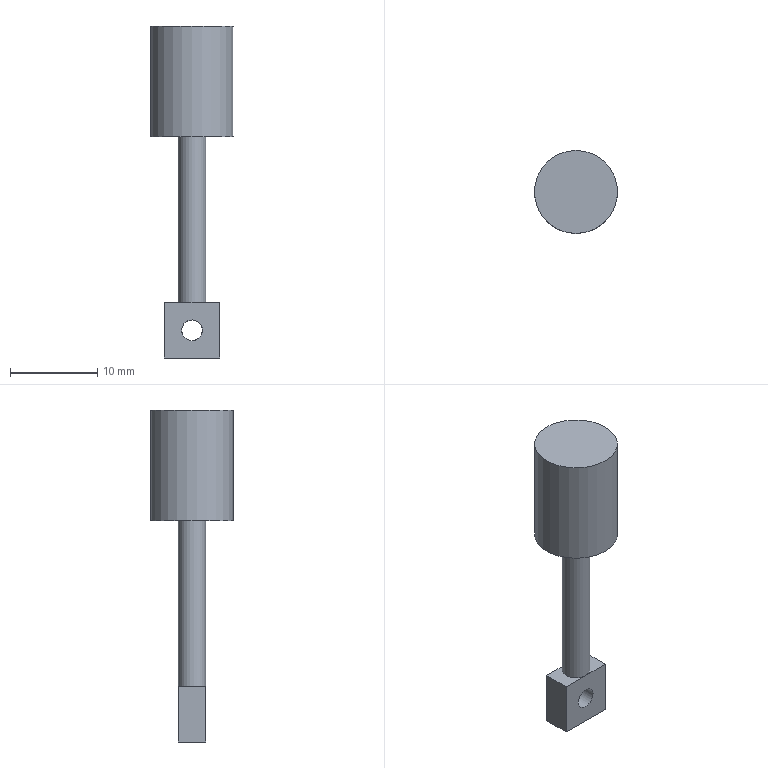Part | NX | features DATUM_CSYS 4, SKETCH 3, EXTRUDE 2, SWP104 1 | 1 solid | 12 faces | box 9.525 x 9.525 x 38.1 mm | volume 1170 mm3 | plane 9 | cylinder 3 | commonest cylinder face diameters 2.381 x1 3.175 x1 9.525 x1
STEP:
#1=CARTESIAN_POINT('',(3.175,1.587,6.35));
#2=VERTEX_POINT('',#1);
#3=CARTESIAN_POINT('',(0.,1.587,6.35));
#4=VERTEX_POINT('',#3);
#5=CARTESIAN_POINT('',(3.175,1.587,6.35));
#6=DIRECTION('',(-1.,0.,0.));
#7=VECTOR('',#6,1000.);
#8=LINE('',#5,#7);
#9=EDGE_CURVE('',#2,#4,#8,.T.);
#10=ORIENTED_EDGE('',*,*,#9,.T.);
#11=CARTESIAN_POINT('',(0.,-1.587,6.35));
#12=VERTEX_POINT('',#11);
#13=CARTESIAN_POINT('',(0.,0.,6.35));
#14=DIRECTION('',(0.,0.,-1.));
#15=DIRECTION('',(0.,1.,0.));
#16=AXIS2_PLACEMENT_3D('',#13,#14,#15);
#17=CIRCLE('',#16,1.587);
#18=EDGE_CURVE('',#4,#12,#17,.T.);
#19=ORIENTED_EDGE('',*,*,#18,.T.);
#20=CARTESIAN_POINT('',(3.175,-1.587,6.35));
#21=VERTEX_POINT('',#20);
#22=CARTESIAN_POINT('',(-3.175,-1.587,6.35));
#23=DIRECTION('',(1.,0.,0.));
#24=VECTOR('',#23,1000.);
#25=LINE('',#22,#24);
#26=EDGE_CURVE('',#12,#21,#25,.T.);
#27=ORIENTED_EDGE('',*,*,#26,.T.);
#28=CARTESIAN_POINT('',(3.175,-1.587,6.35));
#29=DIRECTION('',(0.,1.,0.));
#30=VECTOR('',#29,1000.);
#31=LINE('',#28,#30);
#32=EDGE_CURVE('',#21,#2,#31,.T.);
#33=ORIENTED_EDGE('',*,*,#32,.T.);
#34=EDGE_LOOP('',(#10,#19,#27,#33));
#35=FACE_BOUND('',#34,.T.);
#36=CARTESIAN_POINT('',(0.,0.,6.35));
#37=DIRECTION('',(0.,0.,1.));
#38=DIRECTION('',(1.,0.,0.));
#39=AXIS2_PLACEMENT_3D('',#36,#37,#38);
#40=PLANE('',#39);
#41=ADVANCED_FACE('',(#35),#40,.T.);
#42=CARTESIAN_POINT('',(-3.175,1.587,0.));
#43=VERTEX_POINT('',#42);
#44=CARTESIAN_POINT('',(-3.175,-1.587,0.));
#45=VERTEX_POINT('',#44);
#46=CARTESIAN_POINT('',(-3.175,1.587,0.));
#47=DIRECTION('',(0.,-1.,0.));
#48=VECTOR('',#47,1000.);
#49=LINE('',#46,#48);
#50=EDGE_CURVE('',#43,#45,#49,.T.);
#51=ORIENTED_EDGE('',*,*,#50,.T.);
#52=CARTESIAN_POINT('',(-3.175,-1.587,6.35));
#53=VERTEX_POINT('',#52);
#54=CARTESIAN_POINT('',(-3.175,-1.587,6.35));
#55=DIRECTION('',(0.,0.,-1.));
#56=VECTOR('',#55,1000.);
#57=LINE('',#54,#56);
#58=EDGE_CURVE('',#53,#45,#57,.T.);
#59=ORIENTED_EDGE('',*,*,#58,.F.);
#60=CARTESIAN_POINT('',(-3.175,1.587,6.35));
#61=VERTEX_POINT('',#60);
#62=CARTESIAN_POINT('',(-3.175,1.587,6.35));
#63=DIRECTION('',(0.,-1.,0.));
#64=VECTOR('',#63,1000.);
#65=LINE('',#62,#64);
#66=EDGE_CURVE('',#61,#53,#65,.T.);
#67=ORIENTED_EDGE('',*,*,#66,.F.);
#68=CARTESIAN_POINT('',(-3.175,1.587,6.35));
#69=DIRECTION('',(0.,0.,-1.));
#70=VECTOR('',#69,1000.);
#71=LINE('',#68,#70);
#72=EDGE_CURVE('',#61,#43,#71,.T.);
#73=ORIENTED_EDGE('',*,*,#72,.T.);
#74=EDGE_LOOP('',(#51,#59,#67,#73));
#75=FACE_BOUND('',#74,.T.);
#76=CARTESIAN_POINT('',(-3.175,1.587,6.35));
#77=DIRECTION('',(1.,0.,0.));
#78=DIRECTION('',(0.,0.,-1.));
#79=AXIS2_PLACEMENT_3D('',#76,#77,#78);
#80=PLANE('',#79);
#81=ADVANCED_FACE('',(#75),#80,.F.);
#82=CARTESIAN_POINT('',(1.191,-1.587,3.175));
#83=VERTEX_POINT('',#82);
#84=CARTESIAN_POINT('',(0.,-1.587,3.175));
#85=DIRECTION('',(0.,-1.,0.));
#86=DIRECTION('',(1.,0.,0.));
#87=AXIS2_PLACEMENT_3D('',#84,#85,#86);
#88=CIRCLE('',#87,1.191);
#89=EDGE_CURVE('',#83,#83,#88,.T.);
#90=ORIENTED_EDGE('',*,*,#89,.F.);
#91=EDGE_LOOP('',(#90));
#92=FACE_BOUND('',#91,.T.);
#93=CARTESIAN_POINT('',(3.175,-1.587,0.));
#94=VERTEX_POINT('',#93);
#95=CARTESIAN_POINT('',(-3.175,-1.587,0.));
#96=DIRECTION('',(1.,0.,0.));
#97=VECTOR('',#96,1000.);
#98=LINE('',#95,#97);
#99=EDGE_CURVE('',#45,#94,#98,.T.);
#100=ORIENTED_EDGE('',*,*,#99,.T.);
#101=CARTESIAN_POINT('',(3.175,-1.587,6.35));
#102=DIRECTION('',(0.,0.,-1.));
#103=VECTOR('',#102,1000.);
#104=LINE('',#101,#103);
#105=EDGE_CURVE('',#21,#94,#104,.T.);
#106=ORIENTED_EDGE('',*,*,#105,.F.);
#107=ORIENTED_EDGE('',*,*,#26,.F.);
#108=CARTESIAN_POINT('',(-3.175,-1.587,6.35));
#109=DIRECTION('',(1.,0.,0.));
#110=VECTOR('',#109,1000.);
#111=LINE('',#108,#110);
#112=EDGE_CURVE('',#53,#12,#111,.T.);
#113=ORIENTED_EDGE('',*,*,#112,.F.);
#114=ORIENTED_EDGE('',*,*,#58,.T.);
#115=EDGE_LOOP('',(#100,#106,#107,#113,#114));
#116=FACE_BOUND('',#115,.T.);
#117=CARTESIAN_POINT('',(-3.175,-1.587,6.35));
#118=DIRECTION('',(0.,1.,0.));
#119=DIRECTION('',(0.,0.,1.));
#120=AXIS2_PLACEMENT_3D('',#117,#118,#119);
#121=PLANE('',#120);
#122=ADVANCED_FACE('',(#92,#116),#121,.F.);
#123=CARTESIAN_POINT('',(3.175,1.587,0.));
#124=VERTEX_POINT('',#123);
#125=CARTESIAN_POINT('',(3.175,-1.587,0.));
#126=DIRECTION('',(0.,1.,0.));
#127=VECTOR('',#126,1000.);
#128=LINE('',#125,#127);
#129=EDGE_CURVE('',#94,#124,#128,.T.);
#130=ORIENTED_EDGE('',*,*,#129,.T.);
#131=CARTESIAN_POINT('',(3.175,1.587,6.35));
#132=DIRECTION('',(0.,0.,-1.));
#133=VECTOR('',#132,1000.);
#134=LINE('',#131,#133);
#135=EDGE_CURVE('',#2,#124,#134,.T.);
#136=ORIENTED_EDGE('',*,*,#135,.F.);
#137=ORIENTED_EDGE('',*,*,#32,.F.);
#138=ORIENTED_EDGE('',*,*,#105,.T.);
#139=EDGE_LOOP('',(#130,#136,#137,#138));
#140=FACE_BOUND('',#139,.T.);
#141=CARTESIAN_POINT('',(3.175,-1.587,6.35));
#142=DIRECTION('',(-1.,0.,0.));
#143=DIRECTION('',(0.,0.,1.));
#144=AXIS2_PLACEMENT_3D('',#141,#142,#143);
#145=PLANE('',#144);
#146=ADVANCED_FACE('',(#140),#145,.F.);
#147=CARTESIAN_POINT('',(0.,1.587,1.984));
#148=VERTEX_POINT('',#147);
#149=CARTESIAN_POINT('',(0.,1.587,3.175));
#150=DIRECTION('',(0.,-1.,0.));
#151=DIRECTION('',(0.,0.,-1.));
#152=AXIS2_PLACEMENT_3D('',#149,#150,#151);
#153=CIRCLE('',#152,1.191);
#154=EDGE_CURVE('',#148,#148,#153,.T.);
#155=ORIENTED_EDGE('',*,*,#154,.T.);
#156=EDGE_LOOP('',(#155));
#157=FACE_BOUND('',#156,.T.);
#158=CARTESIAN_POINT('',(3.175,1.587,0.));
#159=DIRECTION('',(-1.,0.,0.));
#160=VECTOR('',#159,1000.);
#161=LINE('',#158,#160);
#162=EDGE_CURVE('',#124,#43,#161,.T.);
#163=ORIENTED_EDGE('',*,*,#162,.T.);
#164=ORIENTED_EDGE('',*,*,#72,.F.);
#165=CARTESIAN_POINT('',(3.175,1.587,6.35));
#166=DIRECTION('',(-1.,0.,0.));
#167=VECTOR('',#166,1000.);
#168=LINE('',#165,#167);
#169=EDGE_CURVE('',#4,#61,#168,.T.);
#170=ORIENTED_EDGE('',*,*,#169,.F.);
#171=ORIENTED_EDGE('',*,*,#9,.F.);
#172=ORIENTED_EDGE('',*,*,#135,.T.);
#173=EDGE_LOOP('',(#163,#164,#170,#171,#172));
#174=FACE_BOUND('',#173,.T.);
#175=CARTESIAN_POINT('',(3.175,1.587,6.35));
#176=DIRECTION('',(0.,-1.,0.));
#177=DIRECTION('',(0.,0.,-1.));
#178=AXIS2_PLACEMENT_3D('',#175,#176,#177);
#179=PLANE('',#178);
#180=ADVANCED_FACE('',(#157,#174),#179,.F.);
#181=ORIENTED_EDGE('',*,*,#112,.T.);
#182=CARTESIAN_POINT('',(0.,0.,6.35));
#183=DIRECTION('',(0.,0.,-1.));
#184=DIRECTION('',(0.,1.,0.));
#185=AXIS2_PLACEMENT_3D('',#182,#183,#184);
#186=CIRCLE('',#185,1.587);
#187=EDGE_CURVE('',#12,#4,#186,.T.);
#188=ORIENTED_EDGE('',*,*,#187,.T.);
#189=ORIENTED_EDGE('',*,*,#169,.T.);
#190=ORIENTED_EDGE('',*,*,#66,.T.);
#191=EDGE_LOOP('',(#181,#188,#189,#190));
#192=FACE_BOUND('',#191,.T.);
#193=CARTESIAN_POINT('',(0.,0.,6.35));
#194=DIRECTION('',(0.,0.,1.));
#195=DIRECTION('',(1.,0.,0.));
#196=AXIS2_PLACEMENT_3D('',#193,#194,#195);
#197=PLANE('',#196);
#198=ADVANCED_FACE('',(#192),#197,.T.);
#199=ORIENTED_EDGE('',*,*,#50,.F.);
#200=ORIENTED_EDGE('',*,*,#162,.F.);
#201=ORIENTED_EDGE('',*,*,#129,.F.);
#202=ORIENTED_EDGE('',*,*,#99,.F.);
#203=EDGE_LOOP('',(#199,#200,#201,#202));
#204=FACE_BOUND('',#203,.T.);
#205=CARTESIAN_POINT('',(0.,0.,0.));
#206=DIRECTION('',(0.,0.,1.));
#207=DIRECTION('',(1.,0.,0.));
#208=AXIS2_PLACEMENT_3D('',#205,#206,#207);
#209=PLANE('',#208);
#210=ADVANCED_FACE('',(#204),#209,.F.);
#211=ORIENTED_EDGE('',*,*,#89,.T.);
#212=EDGE_LOOP('',(#211));
#213=FACE_BOUND('',#212,.T.);
#214=ORIENTED_EDGE('',*,*,#154,.F.);
#215=EDGE_LOOP('',(#214));
#216=FACE_BOUND('',#215,.T.);
#217=CARTESIAN_POINT('',(0.,6.54,3.175));
#218=DIRECTION('',(0.,-1.,0.));
#219=DIRECTION('',(0.,0.,-1.));
#220=AXIS2_PLACEMENT_3D('',#217,#218,#219);
#221=CYLINDRICAL_SURFACE('',#220,1.191);
#222=ADVANCED_FACE('',(#213,#216),#221,.F.);
#223=CARTESIAN_POINT('',(0.,1.587,25.4));
#224=VERTEX_POINT('',#223);
#225=CARTESIAN_POINT('',(0.,0.,25.4));
#226=DIRECTION('',(0.,0.,-1.));
#227=DIRECTION('',(0.,1.,0.));
#228=AXIS2_PLACEMENT_3D('',#225,#226,#227);
#229=CIRCLE('',#228,1.587);
#230=EDGE_CURVE('',#224,#224,#229,.T.);
#231=ORIENTED_EDGE('',*,*,#230,.T.);
#232=EDGE_LOOP('',(#231));
#233=FACE_BOUND('',#232,.T.);
#234=ORIENTED_EDGE('',*,*,#18,.F.);
#235=ORIENTED_EDGE('',*,*,#187,.F.);
#236=EDGE_LOOP('',(#234,#235));
#237=FACE_BOUND('',#236,.T.);
#238=CARTESIAN_POINT('',(0.,0.,38.1));
#239=DIRECTION('',(0.,0.,-1.));
#240=DIRECTION('',(0.,1.,0.));
#241=AXIS2_PLACEMENT_3D('',#238,#239,#240);
#242=CYLINDRICAL_SURFACE('',#241,1.587);
#243=ADVANCED_FACE('',(#233,#237),#242,.T.);
#244=CARTESIAN_POINT('',(0.,4.763,25.4));
#245=VERTEX_POINT('',#244);
#246=CARTESIAN_POINT('',(0.,0.,25.4));
#247=DIRECTION('',(0.,0.,-1.));
#248=DIRECTION('',(0.,1.,0.));
#249=AXIS2_PLACEMENT_3D('',#246,#247,#248);
#250=CIRCLE('',#249,4.763);
#251=EDGE_CURVE('',#245,#245,#250,.T.);
#252=ORIENTED_EDGE('',*,*,#251,.T.);
#253=EDGE_LOOP('',(#252));
#254=FACE_BOUND('',#253,.T.);
#255=ORIENTED_EDGE('',*,*,#230,.F.);
#256=EDGE_LOOP('',(#255));
#257=FACE_BOUND('',#256,.T.);
#258=CARTESIAN_POINT('',(0.,1.587,25.4));
#259=DIRECTION('',(0.,0.,-1.));
#260=DIRECTION('',(0.,1.,0.));
#261=AXIS2_PLACEMENT_3D('',#258,#259,#260);
#262=PLANE('',#261);
#263=ADVANCED_FACE('',(#254,#257),#262,.T.);
#264=CARTESIAN_POINT('',(0.,4.763,38.1));
#265=VERTEX_POINT('',#264);
#266=CARTESIAN_POINT('',(0.,0.,38.1));
#267=DIRECTION('',(0.,0.,-1.));
#268=DIRECTION('',(0.,1.,0.));
#269=AXIS2_PLACEMENT_3D('',#266,#267,#268);
#270=CIRCLE('',#269,4.763);
#271=EDGE_CURVE('',#265,#265,#270,.T.);
#272=ORIENTED_EDGE('',*,*,#271,.T.);
#273=EDGE_LOOP('',(#272));
#274=FACE_BOUND('',#273,.T.);
#275=ORIENTED_EDGE('',*,*,#251,.F.);
#276=EDGE_LOOP('',(#275));
#277=FACE_BOUND('',#276,.T.);
#278=CARTESIAN_POINT('',(0.,0.,38.1));
#279=DIRECTION('',(0.,0.,-1.));
#280=DIRECTION('',(0.,1.,0.));
#281=AXIS2_PLACEMENT_3D('',#278,#279,#280);
#282=CYLINDRICAL_SURFACE('',#281,4.763);
#283=ADVANCED_FACE('',(#274,#277),#282,.T.);
#284=ORIENTED_EDGE('',*,*,#271,.F.);
#285=EDGE_LOOP('',(#284));
#286=FACE_BOUND('',#285,.T.);
#287=CARTESIAN_POINT('',(0.,4.763,38.1));
#288=DIRECTION('',(0.,0.,1.));
#289=DIRECTION('',(0.,-1.,0.));
#290=AXIS2_PLACEMENT_3D('',#287,#288,#289);
#291=PLANE('',#290);
#292=ADVANCED_FACE('',(#286),#291,.T.);
#293=CLOSED_SHELL('',(#41,#81,#122,#146,#180,#198,#210,#222,#243,#263,#283,#292));
#294=MANIFOLD_SOLID_BREP('',#293);
#295=(LENGTH_UNIT()NAMED_UNIT(*)SI_UNIT(.MILLI.,.METRE.));
#296=UNCERTAINTY_MEASURE_WITH_UNIT(LENGTH_MEASURE(0.00001),#295,'','');
#297=(NAMED_UNIT(*)PLANE_ANGLE_UNIT()SI_UNIT($,.RADIAN.));
#298=(NAMED_UNIT(*)SI_UNIT($,.STERADIAN.)SOLID_ANGLE_UNIT());
#299=(GEOMETRIC_REPRESENTATION_CONTEXT(3)GLOBAL_UNCERTAINTY_ASSIGNED_CONTEXT((#296))GLOBAL_UNIT_ASSIGNED_CONTEXT((#295,#297,#298))REPRESENTATION_CONTEXT('',''));
#300=ADVANCED_BREP_SHAPE_REPRESENTATION('',(#294),#299);